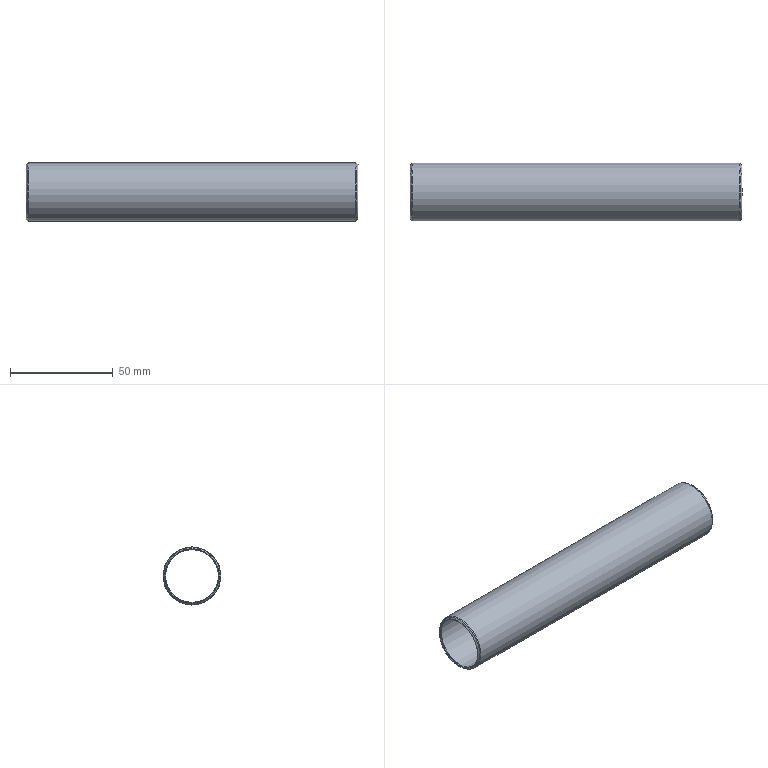Part | NX | features solid 2 | 1 solid | 14 faces | box 161.716 x 28.27 x 28.27 mm | volume 7485 mm3 | cone 6 | cylinder 4 | torus 4 | commonest cylinder face diameters 25.692 x2 27.216 x1 28.27 x1
STEP:
#1=CARTESIAN_POINT('',(0.762,0.,13.608));
#2=VERTEX_POINT('',#1);
#3=CARTESIAN_POINT('',(0.762,0.,0.));
#4=DIRECTION('',(-1.,0.,0.));
#5=DIRECTION('',(0.,0.,1.));
#6=AXIS2_PLACEMENT_3D('',#3,#4,#5);
#7=CIRCLE('',#6,13.608);
#8=EDGE_CURVE('',#2,#2,#7,.T.);
#9=ORIENTED_EDGE('',*,*,#8,.F.);
#10=EDGE_LOOP('',(#9));
#11=FACE_BOUND('',#10,.T.);
#12=CARTESIAN_POINT('',(0.,0.,12.846));
#13=VERTEX_POINT('',#12);
#14=CARTESIAN_POINT('',(0.,0.,0.));
#15=DIRECTION('',(-1.,0.,0.));
#16=DIRECTION('',(0.,0.,1.));
#17=AXIS2_PLACEMENT_3D('',#14,#15,#16);
#18=CIRCLE('',#17,12.846);
#19=EDGE_CURVE('',#13,#13,#18,.T.);
#20=ORIENTED_EDGE('',*,*,#19,.T.);
#21=EDGE_LOOP('',(#20));
#22=FACE_BOUND('',#21,.T.);
#23=CARTESIAN_POINT('',(0.,0.,0.));
#24=DIRECTION('',(1.,0.,0.));
#25=DIRECTION('',(0.,0.,-1.));
#26=AXIS2_PLACEMENT_3D('',#23,#24,#25);
#27=CONICAL_SURFACE('',#26,12.846,0.7854);
#28=ADVANCED_FACE('',(#11,#22),#27,.F.);
#29=CARTESIAN_POINT('',(159.601,0.,13.608));
#30=VERTEX_POINT('',#29);
#31=CARTESIAN_POINT('',(159.601,0.,0.));
#32=DIRECTION('',(-1.,0.,0.));
#33=DIRECTION('',(0.,0.,1.));
#34=AXIS2_PLACEMENT_3D('',#31,#32,#33);
#35=CIRCLE('',#34,13.608);
#36=EDGE_CURVE('',#30,#30,#35,.T.);
#37=ORIENTED_EDGE('',*,*,#36,.F.);
#38=EDGE_LOOP('',(#37));
#39=FACE_BOUND('',#38,.T.);
#40=ORIENTED_EDGE('',*,*,#8,.T.);
#41=EDGE_LOOP('',(#40));
#42=FACE_BOUND('',#41,.T.);
#43=CARTESIAN_POINT('',(160.363,0.,0.));
#44=DIRECTION('',(-1.,0.,0.));
#45=DIRECTION('',(0.,0.,1.));
#46=AXIS2_PLACEMENT_3D('',#43,#44,#45);
#47=CYLINDRICAL_SURFACE('',#46,13.608);
#48=ADVANCED_FACE('',(#39,#42),#47,.F.);
#49=CARTESIAN_POINT('',(160.363,0.,12.846));
#50=VERTEX_POINT('',#49);
#51=CARTESIAN_POINT('',(160.363,0.,0.));
#52=DIRECTION('',(-1.,0.,0.));
#53=DIRECTION('',(0.,0.,1.));
#54=AXIS2_PLACEMENT_3D('',#51,#52,#53);
#55=CIRCLE('',#54,12.846);
#56=EDGE_CURVE('',#50,#50,#55,.T.);
#57=ORIENTED_EDGE('',*,*,#56,.F.);
#58=EDGE_LOOP('',(#57));
#59=FACE_BOUND('',#58,.T.);
#60=ORIENTED_EDGE('',*,*,#36,.T.);
#61=EDGE_LOOP('',(#60));
#62=FACE_BOUND('',#61,.T.);
#63=CARTESIAN_POINT('',(159.601,0.,0.));
#64=DIRECTION('',(-1.,0.,0.));
#65=DIRECTION('',(0.,0.,1.));
#66=AXIS2_PLACEMENT_3D('',#63,#64,#65);
#67=CONICAL_SURFACE('',#66,13.608,0.7854);
#68=ADVANCED_FACE('',(#59,#62),#67,.F.);
#69=CARTESIAN_POINT('',(160.744,0.,12.846));
#70=VERTEX_POINT('',#69);
#71=CARTESIAN_POINT('',(160.744,0.,0.));
#72=DIRECTION('',(-1.,0.,0.));
#73=DIRECTION('',(0.,0.,1.));
#74=AXIS2_PLACEMENT_3D('',#71,#72,#73);
#75=CIRCLE('',#74,12.846);
#76=EDGE_CURVE('',#70,#70,#75,.T.);
#77=ORIENTED_EDGE('',*,*,#76,.F.);
#78=EDGE_LOOP('',(#77));
#79=FACE_BOUND('',#78,.T.);
#80=ORIENTED_EDGE('',*,*,#56,.T.);
#81=EDGE_LOOP('',(#80));
#82=FACE_BOUND('',#81,.T.);
#83=CARTESIAN_POINT('',(160.363,0.,0.));
#84=DIRECTION('',(-1.,0.,0.));
#85=DIRECTION('',(0.,0.,1.));
#86=AXIS2_PLACEMENT_3D('',#83,#84,#85);
#87=CYLINDRICAL_SURFACE('',#86,12.846);
#88=ADVANCED_FACE('',(#79,#82),#87,.F.);
#89=CARTESIAN_POINT('',(161.002,0.,13.105));
#90=VERTEX_POINT('',#89);
#91=CARTESIAN_POINT('',(161.002,0.,0.));
#92=DIRECTION('',(-1.,0.,0.));
#93=DIRECTION('',(0.,0.,1.));
#94=AXIS2_PLACEMENT_3D('',#91,#92,#93);
#95=CIRCLE('',#94,13.105);
#96=EDGE_CURVE('',#90,#90,#95,.T.);
#97=ORIENTED_EDGE('',*,*,#96,.F.);
#98=EDGE_LOOP('',(#97));
#99=FACE_BOUND('',#98,.T.);
#100=ORIENTED_EDGE('',*,*,#76,.T.);
#101=EDGE_LOOP('',(#100));
#102=FACE_BOUND('',#101,.T.);
#103=CARTESIAN_POINT('',(160.744,0.,0.));
#104=DIRECTION('',(1.,0.,0.));
#105=DIRECTION('',(0.,0.,-1.));
#106=AXIS2_PLACEMENT_3D('',#103,#104,#105);
#107=CONICAL_SURFACE('',#106,12.846,0.7854);
#108=ADVANCED_FACE('',(#99,#102),#107,.F.);
#109=ORIENTED_EDGE('',*,*,#96,.T.);
#110=EDGE_LOOP('',(#109));
#111=FACE_BOUND('',#110,.T.);
#112=CARTESIAN_POINT('',(161.002,0.,13.284));
#113=VERTEX_POINT('',#112);
#114=CARTESIAN_POINT('',(161.002,0.,0.));
#115=DIRECTION('',(-1.,0.,0.));
#116=DIRECTION('',(0.,0.,1.));
#117=AXIS2_PLACEMENT_3D('',#114,#115,#116);
#118=CIRCLE('',#117,13.284);
#119=EDGE_CURVE('',#113,#113,#118,.T.);
#120=ORIENTED_EDGE('',*,*,#119,.F.);
#121=EDGE_LOOP('',(#120));
#122=FACE_BOUND('',#121,.T.);
#123=CARTESIAN_POINT('',(160.913,0.,0.));
#124=DIRECTION('',(-1.,0.,0.));
#125=DIRECTION('',(0.,0.,1.));
#126=AXIS2_PLACEMENT_3D('',#123,#124,#125);
#127=TOROIDAL_SURFACE('',#126,13.194,0.127);
#128=ADVANCED_FACE('',(#111,#122),#127,.T.);
#129=CARTESIAN_POINT('',(160.375,0.,13.912));
#130=VERTEX_POINT('',#129);
#131=CARTESIAN_POINT('',(160.375,0.,0.));
#132=DIRECTION('',(-1.,0.,0.));
#133=DIRECTION('',(0.,0.,1.));
#134=AXIS2_PLACEMENT_3D('',#131,#132,#133);
#135=CIRCLE('',#134,13.912);
#136=EDGE_CURVE('',#130,#130,#135,.T.);
#137=ORIENTED_EDGE('',*,*,#136,.F.);
#138=EDGE_LOOP('',(#137));
#139=FACE_BOUND('',#138,.T.);
#140=ORIENTED_EDGE('',*,*,#119,.T.);
#141=EDGE_LOOP('',(#140));
#142=FACE_BOUND('',#141,.T.);
#143=CARTESIAN_POINT('',(161.002,0.,0.));
#144=DIRECTION('',(-1.,0.,0.));
#145=DIRECTION('',(0.,0.,1.));
#146=AXIS2_PLACEMENT_3D('',#143,#144,#145);
#147=CONICAL_SURFACE('',#146,13.284,0.7854);
#148=ADVANCED_FACE('',(#139,#142),#147,.T.);
#149=ORIENTED_EDGE('',*,*,#136,.T.);
#150=EDGE_LOOP('',(#149));
#151=FACE_BOUND('',#150,.T.);
#152=CARTESIAN_POINT('',(159.836,0.,14.135));
#153=VERTEX_POINT('',#152);
#154=CARTESIAN_POINT('',(159.836,0.,0.));
#155=DIRECTION('',(-1.,0.,0.));
#156=DIRECTION('',(0.,0.,1.));
#157=AXIS2_PLACEMENT_3D('',#154,#155,#156);
#158=CIRCLE('',#157,14.135);
#159=EDGE_CURVE('',#153,#153,#158,.T.);
#160=ORIENTED_EDGE('',*,*,#159,.F.);
#161=EDGE_LOOP('',(#160));
#162=FACE_BOUND('',#161,.T.);
#163=CARTESIAN_POINT('',(159.836,0.,0.));
#164=DIRECTION('',(-1.,0.,0.));
#165=DIRECTION('',(0.,0.,1.));
#166=AXIS2_PLACEMENT_3D('',#163,#164,#165);
#167=TOROIDAL_SURFACE('',#166,13.373,0.762);
#168=ADVANCED_FACE('',(#151,#162),#167,.T.);
#169=CARTESIAN_POINT('',(0.527,0.,14.135));
#170=VERTEX_POINT('',#169);
#171=CARTESIAN_POINT('',(0.527,0.,0.));
#172=DIRECTION('',(-1.,0.,0.));
#173=DIRECTION('',(0.,0.,1.));
#174=AXIS2_PLACEMENT_3D('',#171,#172,#173);
#175=CIRCLE('',#174,14.135);
#176=EDGE_CURVE('',#170,#170,#175,.T.);
#177=ORIENTED_EDGE('',*,*,#176,.F.);
#178=EDGE_LOOP('',(#177));
#179=FACE_BOUND('',#178,.T.);
#180=ORIENTED_EDGE('',*,*,#159,.T.);
#181=EDGE_LOOP('',(#180));
#182=FACE_BOUND('',#181,.T.);
#183=CARTESIAN_POINT('',(160.363,0.,0.));
#184=DIRECTION('',(-1.,0.,0.));
#185=DIRECTION('',(0.,0.,1.));
#186=AXIS2_PLACEMENT_3D('',#183,#184,#185);
#187=CYLINDRICAL_SURFACE('',#186,14.135);
#188=ADVANCED_FACE('',(#179,#182),#187,.T.);
#189=ORIENTED_EDGE('',*,*,#176,.T.);
#190=EDGE_LOOP('',(#189));
#191=FACE_BOUND('',#190,.T.);
#192=CARTESIAN_POINT('',(-0.01177,0.,13.912));
#193=VERTEX_POINT('',#192);
#194=CARTESIAN_POINT('',(-0.01177,0.,0.));
#195=DIRECTION('',(-1.,0.,0.));
#196=DIRECTION('',(0.,0.,1.));
#197=AXIS2_PLACEMENT_3D('',#194,#195,#196);
#198=CIRCLE('',#197,13.912);
#199=EDGE_CURVE('',#193,#193,#198,.T.);
#200=ORIENTED_EDGE('',*,*,#199,.F.);
#201=EDGE_LOOP('',(#200));
#202=FACE_BOUND('',#201,.T.);
#203=CARTESIAN_POINT('',(0.527,0.,0.));
#204=DIRECTION('',(-1.,0.,0.));
#205=DIRECTION('',(0.,0.,1.));
#206=AXIS2_PLACEMENT_3D('',#203,#204,#205);
#207=TOROIDAL_SURFACE('',#206,13.373,0.762);
#208=ADVANCED_FACE('',(#191,#202),#207,.T.);
#209=CARTESIAN_POINT('',(-0.6395,0.,13.284));
#210=VERTEX_POINT('',#209);
#211=CARTESIAN_POINT('',(-0.6395,0.,0.));
#212=DIRECTION('',(-1.,0.,0.));
#213=DIRECTION('',(0.,0.,1.));
#214=AXIS2_PLACEMENT_3D('',#211,#212,#213);
#215=CIRCLE('',#214,13.284);
#216=EDGE_CURVE('',#210,#210,#215,.T.);
#217=ORIENTED_EDGE('',*,*,#216,.F.);
#218=EDGE_LOOP('',(#217));
#219=FACE_BOUND('',#218,.T.);
#220=ORIENTED_EDGE('',*,*,#199,.T.);
#221=EDGE_LOOP('',(#220));
#222=FACE_BOUND('',#221,.T.);
#223=CARTESIAN_POINT('',(-0.01177,0.,0.));
#224=DIRECTION('',(1.,0.,0.));
#225=DIRECTION('',(0.,0.,-1.));
#226=AXIS2_PLACEMENT_3D('',#223,#224,#225);
#227=CONICAL_SURFACE('',#226,13.912,0.7854);
#228=ADVANCED_FACE('',(#219,#222),#227,.T.);
#229=ORIENTED_EDGE('',*,*,#216,.T.);
#230=EDGE_LOOP('',(#229));
#231=FACE_BOUND('',#230,.T.);
#232=CARTESIAN_POINT('',(-0.6395,0.,13.105));
#233=VERTEX_POINT('',#232);
#234=CARTESIAN_POINT('',(-0.6395,0.,0.));
#235=DIRECTION('',(-1.,0.,0.));
#236=DIRECTION('',(0.,0.,1.));
#237=AXIS2_PLACEMENT_3D('',#234,#235,#236);
#238=CIRCLE('',#237,13.105);
#239=EDGE_CURVE('',#233,#233,#238,.T.);
#240=ORIENTED_EDGE('',*,*,#239,.F.);
#241=EDGE_LOOP('',(#240));
#242=FACE_BOUND('',#241,.T.);
#243=CARTESIAN_POINT('',(-0.5497,0.,0.));
#244=DIRECTION('',(-1.,0.,0.));
#245=DIRECTION('',(0.,0.,1.));
#246=AXIS2_PLACEMENT_3D('',#243,#244,#245);
#247=TOROIDAL_SURFACE('',#246,13.194,0.127);
#248=ADVANCED_FACE('',(#231,#242),#247,.T.);
#249=CARTESIAN_POINT('',(-0.381,0.,12.846));
#250=VERTEX_POINT('',#249);
#251=CARTESIAN_POINT('',(-0.381,0.,0.));
#252=DIRECTION('',(-1.,0.,0.));
#253=DIRECTION('',(0.,0.,1.));
#254=AXIS2_PLACEMENT_3D('',#251,#252,#253);
#255=CIRCLE('',#254,12.846);
#256=EDGE_CURVE('',#250,#250,#255,.T.);
#257=ORIENTED_EDGE('',*,*,#256,.F.);
#258=EDGE_LOOP('',(#257));
#259=FACE_BOUND('',#258,.T.);
#260=ORIENTED_EDGE('',*,*,#239,.T.);
#261=EDGE_LOOP('',(#260));
#262=FACE_BOUND('',#261,.T.);
#263=CARTESIAN_POINT('',(-0.6395,0.,0.));
#264=DIRECTION('',(-1.,0.,0.));
#265=DIRECTION('',(0.,0.,1.));
#266=AXIS2_PLACEMENT_3D('',#263,#264,#265);
#267=CONICAL_SURFACE('',#266,13.105,0.7854);
#268=ADVANCED_FACE('',(#259,#262),#267,.F.);
#269=ORIENTED_EDGE('',*,*,#19,.F.);
#270=EDGE_LOOP('',(#269));
#271=FACE_BOUND('',#270,.T.);
#272=ORIENTED_EDGE('',*,*,#256,.T.);
#273=EDGE_LOOP('',(#272));
#274=FACE_BOUND('',#273,.T.);
#275=CARTESIAN_POINT('',(160.363,0.,0.));
#276=DIRECTION('',(-1.,0.,0.));
#277=DIRECTION('',(0.,0.,1.));
#278=AXIS2_PLACEMENT_3D('',#275,#276,#277);
#279=CYLINDRICAL_SURFACE('',#278,12.846);
#280=ADVANCED_FACE('',(#271,#274),#279,.F.);
#281=CLOSED_SHELL('',(#28,#48,#68,#88,#108,#128,#148,#168,#188,#208,#228,#248,#268,#280));
#282=MANIFOLD_SOLID_BREP('',#281);
#283=(LENGTH_UNIT()NAMED_UNIT(*)SI_UNIT(.MILLI.,.METRE.));
#284=UNCERTAINTY_MEASURE_WITH_UNIT(LENGTH_MEASURE(0.00001),#283,'','');
#285=(NAMED_UNIT(*)PLANE_ANGLE_UNIT()SI_UNIT($,.RADIAN.));
#286=(NAMED_UNIT(*)SI_UNIT($,.STERADIAN.)SOLID_ANGLE_UNIT());
#287=(GEOMETRIC_REPRESENTATION_CONTEXT(3)GLOBAL_UNCERTAINTY_ASSIGNED_CONTEXT((#284))GLOBAL_UNIT_ASSIGNED_CONTEXT((#283,#285,#286))REPRESENTATION_CONTEXT('',''));
#288=ADVANCED_BREP_SHAPE_REPRESENTATION('',(#282),#287);